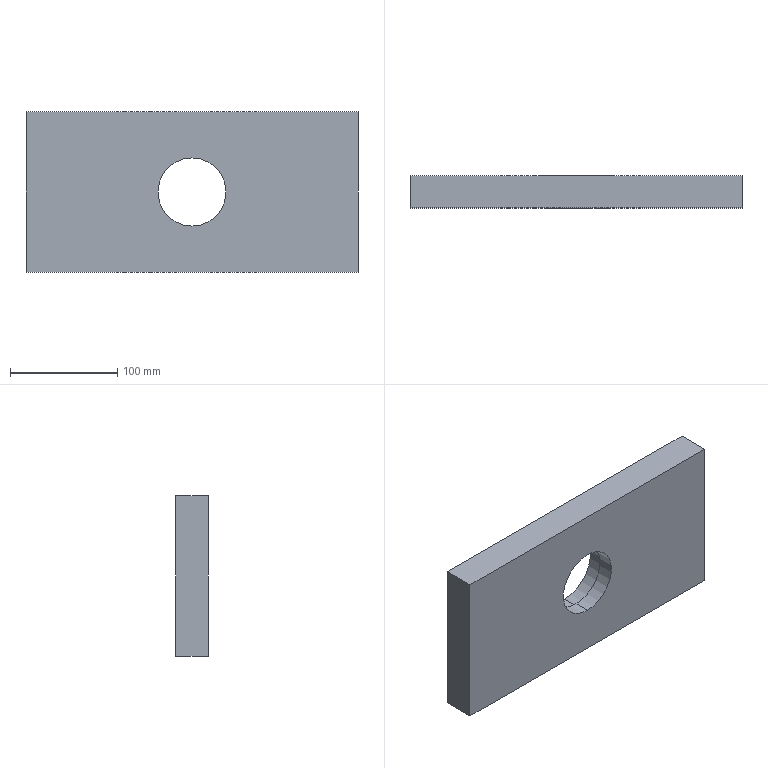Part | SolidWorks | features Cut 2, Extrusion 1 | 1 solid | 11 faces | box 310 x 30 x 150 mm | volume 1293021 mm3 | plane 7 | cylinder 4 | commonest cylinder face diameters 63.5 x2 68 x2
STEP:
#1=CARTESIAN_POINT('',(0.,15.,-34.));
#2=VERTEX_POINT('',#1);
#3=CARTESIAN_POINT('',(0.,15.,34.));
#4=VERTEX_POINT('',#3);
#5=CARTESIAN_POINT('',(0.,15.,0.));
#6=DIRECTION('',(0.,1.,0.));
#7=DIRECTION('',(0.,0.,1.));
#8=AXIS2_PLACEMENT_3D('',#5,#6,#7);
#9=CIRCLE('',#8,34.);
#10=EDGE_CURVE('',#2,#4,#9,.T.);
#11=ORIENTED_EDGE('',*,*,#10,.F.);
#12=CARTESIAN_POINT('',(0.,30.,-34.));
#13=VERTEX_POINT('',#12);
#14=CARTESIAN_POINT('',(0.,15.,-34.));
#15=DIRECTION('',(0.,1.,0.));
#16=VECTOR('',#15,1000.);
#17=LINE('',#14,#16);
#18=EDGE_CURVE('',#2,#13,#17,.T.);
#19=ORIENTED_EDGE('',*,*,#18,.T.);
#20=CARTESIAN_POINT('',(0.,30.,34.));
#21=VERTEX_POINT('',#20);
#22=CARTESIAN_POINT('',(0.,30.,0.));
#23=DIRECTION('',(0.,1.,0.));
#24=DIRECTION('',(0.,0.,1.));
#25=AXIS2_PLACEMENT_3D('',#22,#23,#24);
#26=CIRCLE('',#25,34.);
#27=EDGE_CURVE('',#13,#21,#26,.T.);
#28=ORIENTED_EDGE('',*,*,#27,.T.);
#29=CARTESIAN_POINT('',(0.,15.,34.));
#30=DIRECTION('',(0.,1.,0.));
#31=VECTOR('',#30,1000.);
#32=LINE('',#29,#31);
#33=EDGE_CURVE('',#4,#21,#32,.T.);
#34=ORIENTED_EDGE('',*,*,#33,.F.);
#35=EDGE_LOOP('',(#11,#19,#28,#34));
#36=FACE_OUTER_BOUND('',#35,.T.);
#37=CARTESIAN_POINT('',(0.,15.,0.));
#38=DIRECTION('',(0.,1.,0.));
#39=DIRECTION('',(0.,0.,1.));
#40=AXIS2_PLACEMENT_3D('',#37,#38,#39);
#41=CYLINDRICAL_SURFACE('',#40,34.);
#42=ADVANCED_FACE('',(#36),#41,.F.);
#43=CARTESIAN_POINT('',(0.,0.,-31.75));
#44=VERTEX_POINT('',#43);
#45=CARTESIAN_POINT('',(0.,0.,31.75));
#46=VERTEX_POINT('',#45);
#47=CARTESIAN_POINT('',(0.,0.,0.));
#48=DIRECTION('',(0.,1.,0.));
#49=DIRECTION('',(0.,0.,1.));
#50=AXIS2_PLACEMENT_3D('',#47,#48,#49);
#51=CIRCLE('',#50,31.75);
#52=EDGE_CURVE('',#44,#46,#51,.T.);
#53=ORIENTED_EDGE('',*,*,#52,.F.);
#54=CARTESIAN_POINT('',(0.,15.,-31.75));
#55=VERTEX_POINT('',#54);
#56=CARTESIAN_POINT('',(0.,0.,-31.75));
#57=DIRECTION('',(0.,1.,0.));
#58=VECTOR('',#57,1000.);
#59=LINE('',#56,#58);
#60=EDGE_CURVE('',#44,#55,#59,.T.);
#61=ORIENTED_EDGE('',*,*,#60,.T.);
#62=CARTESIAN_POINT('',(0.,15.,31.75));
#63=VERTEX_POINT('',#62);
#64=CARTESIAN_POINT('',(0.,15.,0.));
#65=DIRECTION('',(0.,-1.,0.));
#66=DIRECTION('',(0.,0.,1.));
#67=AXIS2_PLACEMENT_3D('',#64,#65,#66);
#68=CIRCLE('',#67,31.75);
#69=EDGE_CURVE('',#63,#55,#68,.T.);
#70=ORIENTED_EDGE('',*,*,#69,.F.);
#71=CARTESIAN_POINT('',(0.,0.,31.75));
#72=DIRECTION('',(0.,1.,0.));
#73=VECTOR('',#72,1000.);
#74=LINE('',#71,#73);
#75=EDGE_CURVE('',#46,#63,#74,.T.);
#76=ORIENTED_EDGE('',*,*,#75,.F.);
#77=EDGE_LOOP('',(#53,#61,#70,#76));
#78=FACE_OUTER_BOUND('',#77,.T.);
#79=CARTESIAN_POINT('',(0.,0.,0.));
#80=DIRECTION('',(0.,1.,0.));
#81=DIRECTION('',(0.,0.,1.));
#82=AXIS2_PLACEMENT_3D('',#79,#80,#81);
#83=CYLINDRICAL_SURFACE('',#82,31.75);
#84=ADVANCED_FACE('',(#78),#83,.F.);
#85=ORIENTED_EDGE('',*,*,#60,.F.);
#86=CARTESIAN_POINT('',(0.,0.,0.));
#87=DIRECTION('',(0.,1.,0.));
#88=DIRECTION('',(0.,0.,1.));
#89=AXIS2_PLACEMENT_3D('',#86,#87,#88);
#90=CIRCLE('',#89,31.75);
#91=EDGE_CURVE('',#46,#44,#90,.T.);
#92=ORIENTED_EDGE('',*,*,#91,.F.);
#93=ORIENTED_EDGE('',*,*,#75,.T.);
#94=CARTESIAN_POINT('',(0.,15.,0.));
#95=DIRECTION('',(0.,-1.,0.));
#96=DIRECTION('',(0.,0.,1.));
#97=AXIS2_PLACEMENT_3D('',#94,#95,#96);
#98=CIRCLE('',#97,31.75);
#99=EDGE_CURVE('',#55,#63,#98,.T.);
#100=ORIENTED_EDGE('',*,*,#99,.F.);
#101=EDGE_LOOP('',(#85,#92,#93,#100));
#102=FACE_OUTER_BOUND('',#101,.T.);
#103=CARTESIAN_POINT('',(0.,0.,0.));
#104=DIRECTION('',(0.,1.,0.));
#105=DIRECTION('',(0.,0.,1.));
#106=AXIS2_PLACEMENT_3D('',#103,#104,#105);
#107=CYLINDRICAL_SURFACE('',#106,31.75);
#108=ADVANCED_FACE('',(#102),#107,.F.);
#109=CARTESIAN_POINT('',(155.,0.,75.));
#110=VERTEX_POINT('',#109);
#111=CARTESIAN_POINT('',(155.,0.,-75.));
#112=VERTEX_POINT('',#111);
#113=CARTESIAN_POINT('',(155.,0.,75.));
#114=DIRECTION('',(0.,0.,-1.));
#115=VECTOR('',#114,1000.);
#116=LINE('',#113,#115);
#117=EDGE_CURVE('',#110,#112,#116,.T.);
#118=ORIENTED_EDGE('',*,*,#117,.T.);
#119=CARTESIAN_POINT('',(155.,30.,-75.));
#120=VERTEX_POINT('',#119);
#121=CARTESIAN_POINT('',(155.,30.,-75.));
#122=DIRECTION('',(0.,-1.,0.));
#123=VECTOR('',#122,1000.);
#124=LINE('',#121,#123);
#125=EDGE_CURVE('',#120,#112,#124,.T.);
#126=ORIENTED_EDGE('',*,*,#125,.F.);
#127=CARTESIAN_POINT('',(155.,30.,75.));
#128=VERTEX_POINT('',#127);
#129=CARTESIAN_POINT('',(155.,30.,75.));
#130=DIRECTION('',(0.,0.,-1.));
#131=VECTOR('',#130,1000.);
#132=LINE('',#129,#131);
#133=EDGE_CURVE('',#128,#120,#132,.T.);
#134=ORIENTED_EDGE('',*,*,#133,.F.);
#135=CARTESIAN_POINT('',(155.,30.,75.));
#136=DIRECTION('',(0.,-1.,0.));
#137=VECTOR('',#136,1000.);
#138=LINE('',#135,#137);
#139=EDGE_CURVE('',#128,#110,#138,.T.);
#140=ORIENTED_EDGE('',*,*,#139,.T.);
#141=EDGE_LOOP('',(#118,#126,#134,#140));
#142=FACE_OUTER_BOUND('',#141,.T.);
#143=CARTESIAN_POINT('',(155.,30.,75.));
#144=DIRECTION('',(-1.,0.,0.));
#145=DIRECTION('',(0.,0.,1.));
#146=AXIS2_PLACEMENT_3D('',#143,#144,#145);
#147=PLANE('',#146);
#148=ADVANCED_FACE('',(#142),#147,.F.);
#149=CARTESIAN_POINT('',(-155.,0.,-75.));
#150=VERTEX_POINT('',#149);
#151=CARTESIAN_POINT('',(-155.,0.,-75.));
#152=DIRECTION('',(-1.,0.,0.));
#153=VECTOR('',#152,1000.);
#154=LINE('',#151,#153);
#155=EDGE_CURVE('',#112,#150,#154,.T.);
#156=ORIENTED_EDGE('',*,*,#155,.T.);
#157=CARTESIAN_POINT('',(-155.,30.,-75.));
#158=VERTEX_POINT('',#157);
#159=CARTESIAN_POINT('',(-155.,30.,-75.));
#160=DIRECTION('',(0.,-1.,0.));
#161=VECTOR('',#160,1000.);
#162=LINE('',#159,#161);
#163=EDGE_CURVE('',#158,#150,#162,.T.);
#164=ORIENTED_EDGE('',*,*,#163,.F.);
#165=CARTESIAN_POINT('',(-155.,30.,-75.));
#166=DIRECTION('',(-1.,0.,0.));
#167=VECTOR('',#166,1000.);
#168=LINE('',#165,#167);
#169=EDGE_CURVE('',#120,#158,#168,.T.);
#170=ORIENTED_EDGE('',*,*,#169,.F.);
#171=ORIENTED_EDGE('',*,*,#125,.T.);
#172=EDGE_LOOP('',(#156,#164,#170,#171));
#173=FACE_OUTER_BOUND('',#172,.T.);
#174=CARTESIAN_POINT('',(-155.,30.,-75.));
#175=DIRECTION('',(0.,0.,1.));
#176=DIRECTION('',(1.,0.,0.));
#177=AXIS2_PLACEMENT_3D('',#174,#175,#176);
#178=PLANE('',#177);
#179=ADVANCED_FACE('',(#173),#178,.F.);
#180=CARTESIAN_POINT('',(-155.,0.,75.));
#181=VERTEX_POINT('',#180);
#182=CARTESIAN_POINT('',(-155.,0.,75.));
#183=DIRECTION('',(0.,0.,1.));
#184=VECTOR('',#183,1000.);
#185=LINE('',#182,#184);
#186=EDGE_CURVE('',#150,#181,#185,.T.);
#187=ORIENTED_EDGE('',*,*,#186,.T.);
#188=CARTESIAN_POINT('',(-155.,30.,75.));
#189=VERTEX_POINT('',#188);
#190=CARTESIAN_POINT('',(-155.,30.,75.));
#191=DIRECTION('',(0.,-1.,0.));
#192=VECTOR('',#191,1000.);
#193=LINE('',#190,#192);
#194=EDGE_CURVE('',#189,#181,#193,.T.);
#195=ORIENTED_EDGE('',*,*,#194,.F.);
#196=CARTESIAN_POINT('',(-155.,30.,75.));
#197=DIRECTION('',(0.,0.,1.));
#198=VECTOR('',#197,1000.);
#199=LINE('',#196,#198);
#200=EDGE_CURVE('',#158,#189,#199,.T.);
#201=ORIENTED_EDGE('',*,*,#200,.F.);
#202=ORIENTED_EDGE('',*,*,#163,.T.);
#203=EDGE_LOOP('',(#187,#195,#201,#202));
#204=FACE_OUTER_BOUND('',#203,.T.);
#205=CARTESIAN_POINT('',(-155.,30.,75.));
#206=DIRECTION('',(1.,0.,0.));
#207=DIRECTION('',(0.,0.,-1.));
#208=AXIS2_PLACEMENT_3D('',#205,#206,#207);
#209=PLANE('',#208);
#210=ADVANCED_FACE('',(#204),#209,.F.);
#211=CARTESIAN_POINT('',(-155.,0.,75.));
#212=DIRECTION('',(1.,0.,0.));
#213=VECTOR('',#212,1000.);
#214=LINE('',#211,#213);
#215=EDGE_CURVE('',#181,#110,#214,.T.);
#216=ORIENTED_EDGE('',*,*,#215,.T.);
#217=ORIENTED_EDGE('',*,*,#139,.F.);
#218=CARTESIAN_POINT('',(-155.,30.,75.));
#219=DIRECTION('',(1.,0.,0.));
#220=VECTOR('',#219,1000.);
#221=LINE('',#218,#220);
#222=EDGE_CURVE('',#189,#128,#221,.T.);
#223=ORIENTED_EDGE('',*,*,#222,.F.);
#224=ORIENTED_EDGE('',*,*,#194,.T.);
#225=EDGE_LOOP('',(#216,#217,#223,#224));
#226=FACE_OUTER_BOUND('',#225,.T.);
#227=CARTESIAN_POINT('',(-155.,30.,75.));
#228=DIRECTION('',(0.,0.,-1.));
#229=DIRECTION('',(-1.,0.,0.));
#230=AXIS2_PLACEMENT_3D('',#227,#228,#229);
#231=PLANE('',#230);
#232=ADVANCED_FACE('',(#226),#231,.F.);
#233=CARTESIAN_POINT('',(0.,30.,0.));
#234=DIRECTION('',(0.,1.,0.));
#235=DIRECTION('',(0.,0.,1.));
#236=AXIS2_PLACEMENT_3D('',#233,#234,#235);
#237=CIRCLE('',#236,34.);
#238=EDGE_CURVE('',#21,#13,#237,.T.);
#239=ORIENTED_EDGE('',*,*,#238,.F.);
#240=ORIENTED_EDGE('',*,*,#27,.F.);
#241=EDGE_LOOP('',(#239,#240));
#242=FACE_BOUND('',#241,.T.);
#243=ORIENTED_EDGE('',*,*,#133,.T.);
#244=ORIENTED_EDGE('',*,*,#169,.T.);
#245=ORIENTED_EDGE('',*,*,#200,.T.);
#246=ORIENTED_EDGE('',*,*,#222,.T.);
#247=EDGE_LOOP('',(#243,#244,#245,#246));
#248=FACE_OUTER_BOUND('',#247,.T.);
#249=CARTESIAN_POINT('',(0.,30.,0.));
#250=DIRECTION('',(0.,-1.,0.));
#251=DIRECTION('',(0.,0.,-1.));
#252=AXIS2_PLACEMENT_3D('',#249,#250,#251);
#253=PLANE('',#252);
#254=ADVANCED_FACE('',(#242,#248),#253,.F.);
#255=ORIENTED_EDGE('',*,*,#91,.T.);
#256=ORIENTED_EDGE('',*,*,#52,.T.);
#257=EDGE_LOOP('',(#255,#256));
#258=FACE_BOUND('',#257,.T.);
#259=ORIENTED_EDGE('',*,*,#117,.F.);
#260=ORIENTED_EDGE('',*,*,#215,.F.);
#261=ORIENTED_EDGE('',*,*,#186,.F.);
#262=ORIENTED_EDGE('',*,*,#155,.F.);
#263=EDGE_LOOP('',(#259,#260,#261,#262));
#264=FACE_OUTER_BOUND('',#263,.T.);
#265=CARTESIAN_POINT('',(0.,0.,0.));
#266=DIRECTION('',(0.,-1.,0.));
#267=DIRECTION('',(0.,0.,-1.));
#268=AXIS2_PLACEMENT_3D('',#265,#266,#267);
#269=PLANE('',#268);
#270=ADVANCED_FACE('',(#258,#264),#269,.T.);
#271=CARTESIAN_POINT('',(0.,15.,0.));
#272=DIRECTION('',(0.,1.,0.));
#273=DIRECTION('',(0.,0.,1.));
#274=AXIS2_PLACEMENT_3D('',#271,#272,#273);
#275=CIRCLE('',#274,34.);
#276=EDGE_CURVE('',#4,#2,#275,.T.);
#277=ORIENTED_EDGE('',*,*,#276,.T.);
#278=ORIENTED_EDGE('',*,*,#10,.T.);
#279=EDGE_LOOP('',(#277,#278));
#280=FACE_OUTER_BOUND('',#279,.T.);
#281=ORIENTED_EDGE('',*,*,#69,.T.);
#282=ORIENTED_EDGE('',*,*,#99,.T.);
#283=EDGE_LOOP('',(#281,#282));
#284=FACE_BOUND('',#283,.T.);
#285=CARTESIAN_POINT('',(0.,15.,0.));
#286=DIRECTION('',(0.,1.,0.));
#287=DIRECTION('',(0.,0.,1.));
#288=AXIS2_PLACEMENT_3D('',#285,#286,#287);
#289=PLANE('',#288);
#290=ADVANCED_FACE('',(#280,#284),#289,.T.);
#291=ORIENTED_EDGE('',*,*,#18,.F.);
#292=ORIENTED_EDGE('',*,*,#276,.F.);
#293=ORIENTED_EDGE('',*,*,#33,.T.);
#294=ORIENTED_EDGE('',*,*,#238,.T.);
#295=EDGE_LOOP('',(#291,#292,#293,#294));
#296=FACE_OUTER_BOUND('',#295,.T.);
#297=CARTESIAN_POINT('',(0.,15.,0.));
#298=DIRECTION('',(0.,1.,0.));
#299=DIRECTION('',(0.,0.,1.));
#300=AXIS2_PLACEMENT_3D('',#297,#298,#299);
#301=CYLINDRICAL_SURFACE('',#300,34.);
#302=ADVANCED_FACE('',(#296),#301,.F.);
#303=CLOSED_SHELL('',(#42,#84,#108,#148,#179,#210,#232,#254,#270,#290,#302));
#304=MANIFOLD_SOLID_BREP('',#303);
#305=CARTESIAN_POINT('',(0.,0.,0.));
#306=DIRECTION('',(0.,0.,1.));
#307=DIRECTION('',(1.,0.,0.));
#308=AXIS2_PLACEMENT_3D('',#305,#306,#307);
#309=(LENGTH_UNIT()NAMED_UNIT(*)SI_UNIT(.MILLI.,.METRE.));
#310=UNCERTAINTY_MEASURE_WITH_UNIT(LENGTH_MEASURE(0.00001),#309,'','');
#311=(NAMED_UNIT(*)PLANE_ANGLE_UNIT()SI_UNIT($,.RADIAN.));
#312=(NAMED_UNIT(*)SI_UNIT($,.STERADIAN.)SOLID_ANGLE_UNIT());
#313=(GEOMETRIC_REPRESENTATION_CONTEXT(3)GLOBAL_UNCERTAINTY_ASSIGNED_CONTEXT((#310))GLOBAL_UNIT_ASSIGNED_CONTEXT((#309,#311,#312))REPRESENTATION_CONTEXT('',''));
#314=ADVANCED_BREP_SHAPE_REPRESENTATION('',(#304,#308),#313);